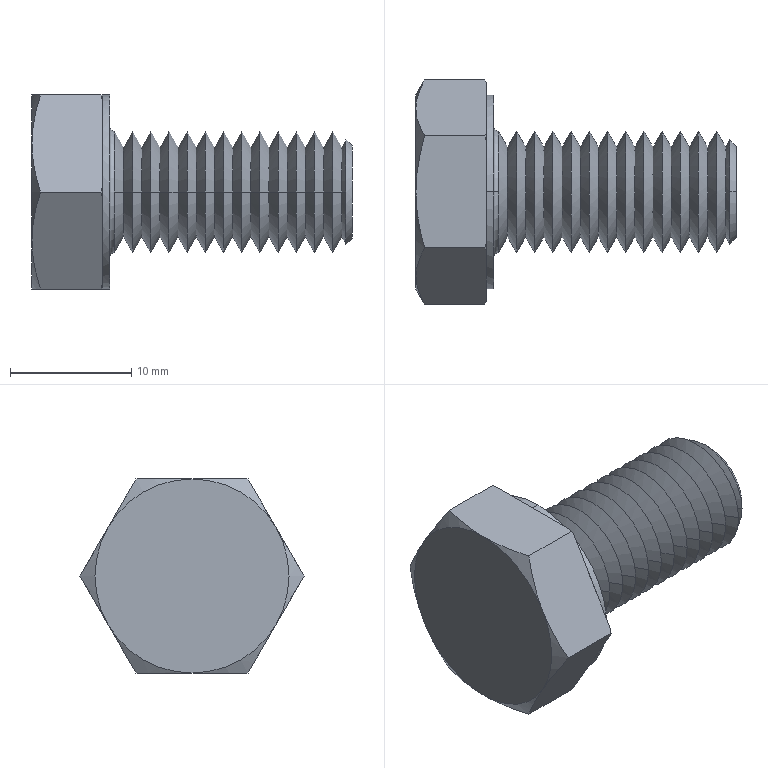Part | SolidWorks | features RevCut 4, Chamfer 1, Extrusion 1, Fillet 1, LPattern 1, Revolution 1 | 1 solid | 109 faces | box 26.4 x 18.475 x 16 mm | volume 2601 mm3 | cone 66 | cylinder 26 | plane 15 | torus 2 | commonest cylinder face diameters 10 x24 16 x2